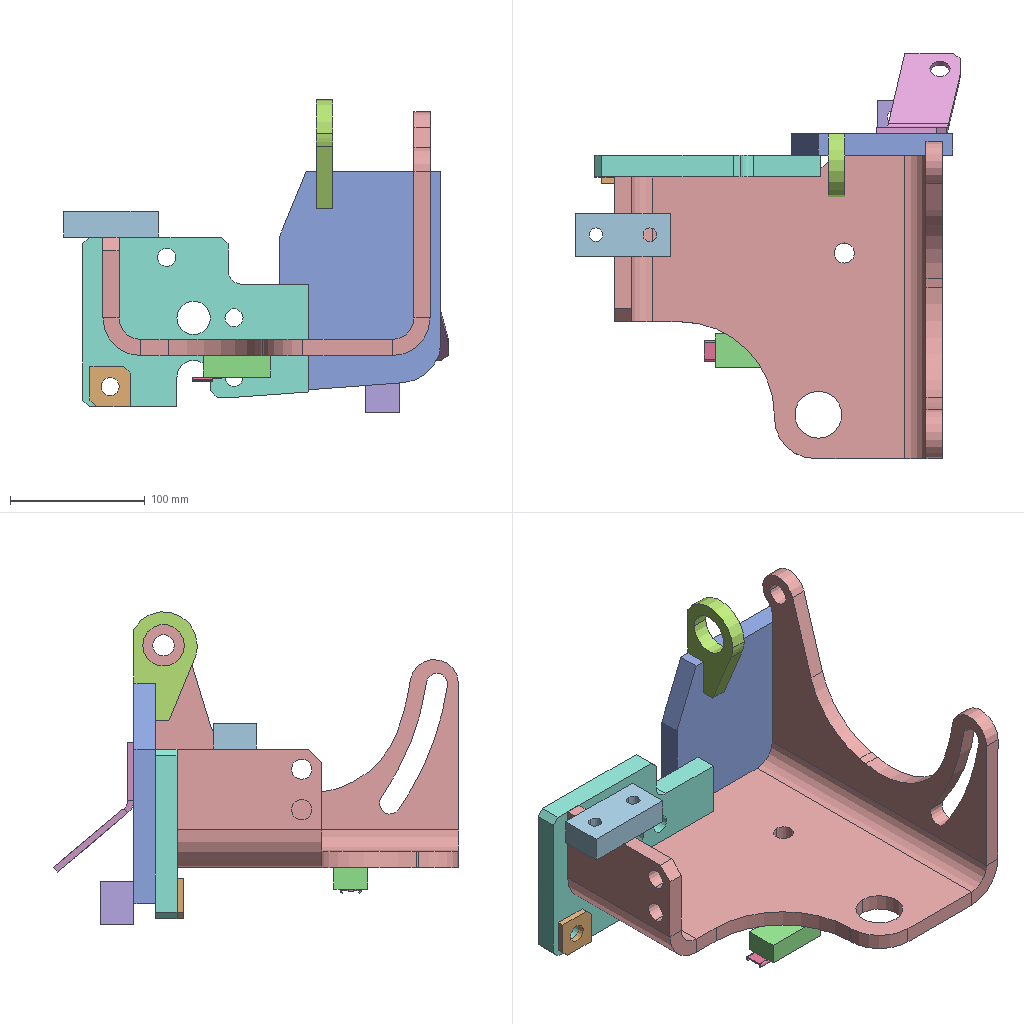Assembly | SolidWorks | 10 different items | 10 placed | box 285 x 301 x 232 mm
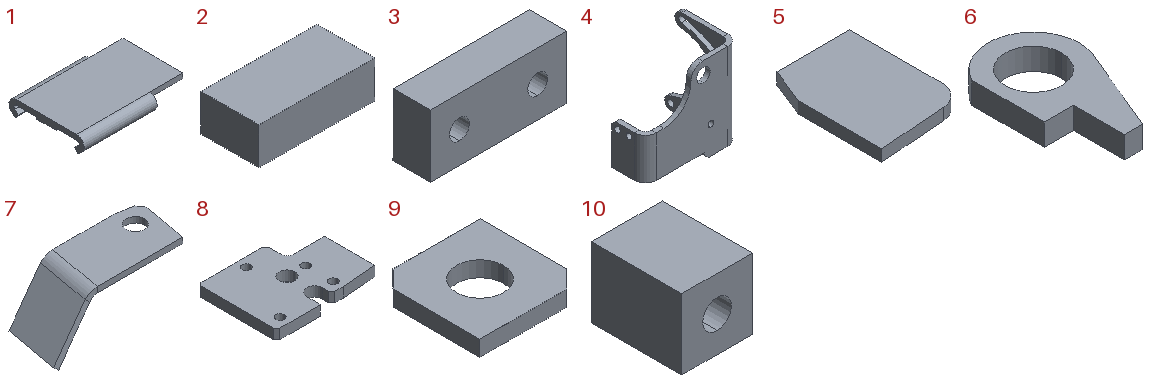Parts list (item | quantity | size | volume | features):
1 | x1 | 22 x 15.54 x 3.327 mm | 392.885 mm3 | features ICE 8, EdgeFlange 2, Hem 2, FlatPattern 1, SMBaseFlange 1, SheetMetal 1
2 | x1 | 50 x 25 x 16 mm | 20000 mm3 | features FlatPattern 1, SMBaseFlange 1, SheetMetal 1
3 | x1 | 70 x 19 x 32 mm | 39455 mm3 | features FlatPattern 1, HoleWzd 1, SMBaseFlange 1, SheetMetal 1
4 | x1 | 243 x 181 x 235 mm | 751047 mm3 | features ICE 3, Chamfer 1, Fillet 1, FlatPattern 1, SMBaseFlange 1, SheetMetal 1
5 | x1 | 120 x 164 x 16 mm | 295810 mm3 | features FlatPattern 1, SMBaseFlange 1, SheetMetal 1
6 | x1 | 47 x 81 x 12 mm | 22191 mm3 | features FlatPattern 1, SMBaseFlange 1, SheetMetal 1
7 | x1 | 113.633 x 47.299 x 39.859 mm | 23066 mm3 | features FlatPattern 1, SM3dBend 1, SMBaseFlange 1, SheetMetal 1
8 | x1 | 168 x 126 x 16 mm | 264942 mm3 | features FlatPattern 1, SMBaseFlange 1, SheetMetal 1
9 | x1 | 30 x 30 x 4.5 mm | 3293 mm3 | features FlatPattern 1, SMBaseFlange 1, SheetMetal 1
10 | x1 | 25 x 32 x 25 mm | 17385 mm3 | features Extrusion 1, HoleWzd 1
Mates (type | each side: item.copy, entity, surface, feature):
Coincident | 4.1 face plane Cut-Extrude1 | 5.1 face plane Base-Flange1
DistanceDim | 4.1 face plane Base-Flange1 | 5.1 face plane Base-Flange1
DistanceDim | 4.1 face cylinder Cut-Extrude1 | 5.1 face plane Base-Flange1
Coincident | 5.1 face plane Base-Flange1 | 6.1 face plane Base-Flange1 | 2 times
DistanceDim | 4.1 face plane Base-Flange1 | 6.1 face plane Base-Flange1
Coincident | 5.1 face plane Base-Flange1 | 7.1 face plane Base-Flange1
Coincident | 4.1 face plane Cut-Extrude2 | 8.1 face plane Base-Flange1 | 2 times
Coincident | 4.1 face plane Base-Flange1 | 8.1 face plane Base-Flange1
Coincident | 8.1 face plane Base-Flange1 | 9.1 face plane Base-Flange1 | 2 times
Concentric | 8.1 face cylinder Base-Flange1 | 9.1 face cylinder Base-Flange1
Coincident | 5.1 face plane Base-Flange1 | 10.1 face plane Boss-Extrude1
DistanceDim | 4.1 face cylinder Cut-Extrude2 | 10.1 face plane Boss-Extrude1
DistanceDim | 8.1 face cylinder Base-Flange1 | 10.1 face plane Boss-Extrude1
DistanceDim | 10.1 face plane Boss-Extrude1 | 7.1 face plane Base-Flange1
DistanceDim | 10.1 face plane Boss-Extrude1 | 7.1 edge
Coincident | 4.1 face plane Base-Flange1 | 2.1 face plane Base-Flange1
DistanceDim | 4.1 face cylinder Cut-Extrude2 | 2.1 face plane Base-Flange1 | 2 times
Parallel | 2.1 face plane Base-Flange1 | assembly plane
Coincident | 2.1 face plane Base-Flange1 | 1.1 face plane Edge-Flange2
DistanceDim | 2.1 face plane Base-Flange1 | 1.1 face plane Cut-Extrude12
DistanceDim | 2.1 face plane Base-Flange1 | 1.1 edge
Coincident | 4.1 face plane Base-Flange1 | 3.1 face plane Base-Flange1
DistanceDim | 8.1 face plane Base-Flange1 | 3.1 face plane Base-Flange1
DistanceDim | 8.1 face cylinder Base-Flange1 | 3.1 face plane Base-Flange1